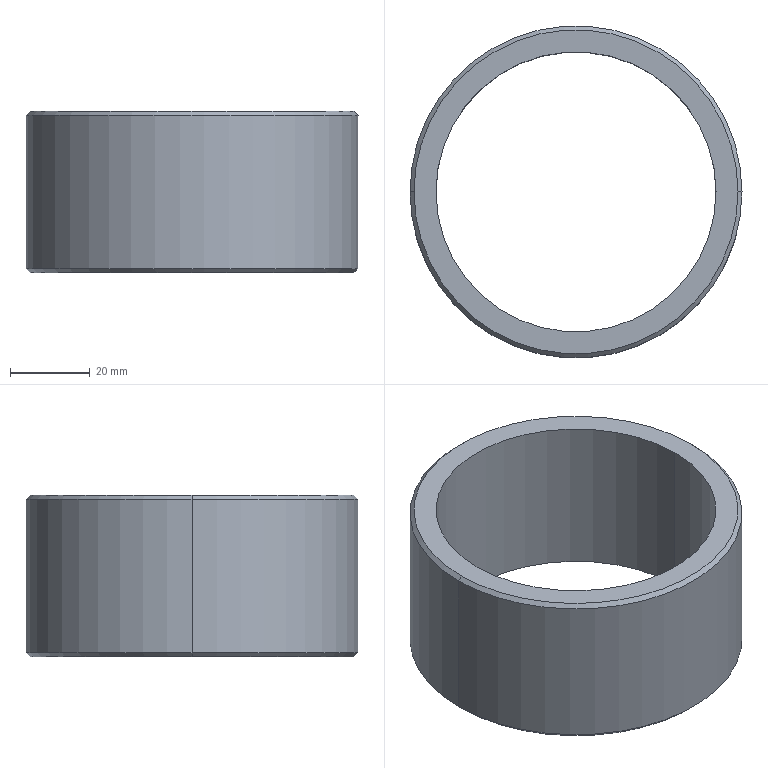Part | SolidWorks | features Chamfer 1, Extrusion 1 | 1 solid | 10 faces | box 83 x 83 x 40.5 mm | volume 63009 mm3 | cone 4 | cylinder 4 | plane 2 | commonest cylinder face diameters 70 x2 83 x2
STEP:
#1=CARTESIAN_POINT('',(40.5,0.,40.5));
#2=VERTEX_POINT('',#1);
#3=CARTESIAN_POINT('',(-40.5,0.,40.5));
#4=VERTEX_POINT('',#3);
#5=CARTESIAN_POINT('',(0.,0.,40.5));
#6=DIRECTION('',(0.,0.,1.));
#7=DIRECTION('',(1.,0.,0.));
#8=AXIS2_PLACEMENT_3D('',#5,#6,#7);
#9=CIRCLE('',#8,40.5);
#10=EDGE_CURVE('',#2,#4,#9,.T.);
#11=ORIENTED_EDGE('',*,*,#10,.F.);
#12=CARTESIAN_POINT('',(41.5,0.,39.5));
#13=VERTEX_POINT('',#12);
#14=CARTESIAN_POINT('',(40.5,0.,40.5));
#15=DIRECTION('',(0.7071,0.,-0.7071));
#16=VECTOR('',#15,1000.);
#17=LINE('',#14,#16);
#18=EDGE_CURVE('',#2,#13,#17,.T.);
#19=ORIENTED_EDGE('',*,*,#18,.T.);
#20=CARTESIAN_POINT('',(-41.5,0.,39.5));
#21=VERTEX_POINT('',#20);
#22=CARTESIAN_POINT('',(0.,0.,39.5));
#23=DIRECTION('',(0.,0.,-1.));
#24=DIRECTION('',(1.,0.,0.));
#25=AXIS2_PLACEMENT_3D('',#22,#23,#24);
#26=CIRCLE('',#25,41.5);
#27=EDGE_CURVE('',#21,#13,#26,.T.);
#28=ORIENTED_EDGE('',*,*,#27,.F.);
#29=CARTESIAN_POINT('',(-40.5,0.,40.5));
#30=DIRECTION('',(-0.7071,0.,-0.7071));
#31=VECTOR('',#30,1000.);
#32=LINE('',#29,#31);
#33=EDGE_CURVE('',#4,#21,#32,.T.);
#34=ORIENTED_EDGE('',*,*,#33,.F.);
#35=EDGE_LOOP('',(#11,#19,#28,#34));
#36=FACE_OUTER_BOUND('',#35,.T.);
#37=CARTESIAN_POINT('',(0.,0.,40.5));
#38=DIRECTION('',(0.,0.,-1.));
#39=DIRECTION('',(-1.,0.,0.));
#40=AXIS2_PLACEMENT_3D('',#37,#38,#39);
#41=CONICAL_SURFACE('',#40,40.5,0.7854);
#42=ADVANCED_FACE('',(#36),#41,.T.);
#43=CARTESIAN_POINT('',(-40.5,0.,0.));
#44=VERTEX_POINT('',#43);
#45=CARTESIAN_POINT('',(40.5,0.,0.));
#46=VERTEX_POINT('',#45);
#47=CARTESIAN_POINT('',(0.,0.,0.));
#48=DIRECTION('',(0.,0.,-1.));
#49=DIRECTION('',(1.,0.,0.));
#50=AXIS2_PLACEMENT_3D('',#47,#48,#49);
#51=CIRCLE('',#50,40.5);
#52=EDGE_CURVE('',#44,#46,#51,.T.);
#53=ORIENTED_EDGE('',*,*,#52,.F.);
#54=CARTESIAN_POINT('',(-41.5,0.,1.));
#55=VERTEX_POINT('',#54);
#56=CARTESIAN_POINT('',(-41.5,0.,1.));
#57=DIRECTION('',(-0.7071,0.,0.7071));
#58=VECTOR('',#57,1000.);
#59=LINE('',#56,#58);
#60=EDGE_CURVE('',#44,#55,#59,.T.);
#61=ORIENTED_EDGE('',*,*,#60,.T.);
#62=CARTESIAN_POINT('',(41.5,0.,1.));
#63=VERTEX_POINT('',#62);
#64=CARTESIAN_POINT('',(0.,0.,1.));
#65=DIRECTION('',(0.,0.,1.));
#66=DIRECTION('',(1.,0.,0.));
#67=AXIS2_PLACEMENT_3D('',#64,#65,#66);
#68=CIRCLE('',#67,41.5);
#69=EDGE_CURVE('',#63,#55,#68,.T.);
#70=ORIENTED_EDGE('',*,*,#69,.F.);
#71=CARTESIAN_POINT('',(41.5,0.,1.));
#72=DIRECTION('',(0.7071,0.,0.7071));
#73=VECTOR('',#72,1000.);
#74=LINE('',#71,#73);
#75=EDGE_CURVE('',#46,#63,#74,.T.);
#76=ORIENTED_EDGE('',*,*,#75,.F.);
#77=EDGE_LOOP('',(#53,#61,#70,#76));
#78=FACE_OUTER_BOUND('',#77,.T.);
#79=CARTESIAN_POINT('',(0.,0.,1.));
#80=DIRECTION('',(0.,0.,1.));
#81=DIRECTION('',(1.,0.,0.));
#82=AXIS2_PLACEMENT_3D('',#79,#80,#81);
#83=CONICAL_SURFACE('',#82,41.5,0.7854);
#84=ADVANCED_FACE('',(#78),#83,.T.);
#85=CARTESIAN_POINT('',(-35.,0.,40.5));
#86=VERTEX_POINT('',#85);
#87=CARTESIAN_POINT('',(35.,0.,40.5));
#88=VERTEX_POINT('',#87);
#89=CARTESIAN_POINT('',(0.,0.,40.5));
#90=DIRECTION('',(0.,0.,1.));
#91=DIRECTION('',(1.,0.,0.));
#92=AXIS2_PLACEMENT_3D('',#89,#90,#91);
#93=CIRCLE('',#92,35.);
#94=EDGE_CURVE('',#86,#88,#93,.T.);
#95=ORIENTED_EDGE('',*,*,#94,.T.);
#96=CARTESIAN_POINT('',(35.,0.,0.));
#97=VERTEX_POINT('',#96);
#98=CARTESIAN_POINT('',(35.,0.,40.5));
#99=DIRECTION('',(0.,0.,-1.));
#100=VECTOR('',#99,1000.);
#101=LINE('',#98,#100);
#102=EDGE_CURVE('',#88,#97,#101,.T.);
#103=ORIENTED_EDGE('',*,*,#102,.T.);
#104=CARTESIAN_POINT('',(-35.,0.,0.));
#105=VERTEX_POINT('',#104);
#106=CARTESIAN_POINT('',(0.,0.,0.));
#107=DIRECTION('',(0.,0.,1.));
#108=DIRECTION('',(1.,0.,0.));
#109=AXIS2_PLACEMENT_3D('',#106,#107,#108);
#110=CIRCLE('',#109,35.);
#111=EDGE_CURVE('',#105,#97,#110,.T.);
#112=ORIENTED_EDGE('',*,*,#111,.F.);
#113=CARTESIAN_POINT('',(-35.,0.,40.5));
#114=DIRECTION('',(0.,0.,-1.));
#115=VECTOR('',#114,1000.);
#116=LINE('',#113,#115);
#117=EDGE_CURVE('',#86,#105,#116,.T.);
#118=ORIENTED_EDGE('',*,*,#117,.F.);
#119=EDGE_LOOP('',(#95,#103,#112,#118));
#120=FACE_OUTER_BOUND('',#119,.T.);
#121=CARTESIAN_POINT('',(0.,0.,40.5));
#122=DIRECTION('',(0.,0.,-1.));
#123=DIRECTION('',(-1.,0.,0.));
#124=AXIS2_PLACEMENT_3D('',#121,#122,#123);
#125=CYLINDRICAL_SURFACE('',#124,35.);
#126=ADVANCED_FACE('',(#120),#125,.F.);
#127=ORIENTED_EDGE('',*,*,#27,.T.);
#128=CARTESIAN_POINT('',(41.5,0.,40.5));
#129=DIRECTION('',(0.,0.,-1.));
#130=VECTOR('',#129,1000.);
#131=LINE('',#128,#130);
#132=EDGE_CURVE('',#13,#63,#131,.T.);
#133=ORIENTED_EDGE('',*,*,#132,.T.);
#134=ORIENTED_EDGE('',*,*,#69,.T.);
#135=CARTESIAN_POINT('',(-41.5,0.,40.5));
#136=DIRECTION('',(0.,0.,-1.));
#137=VECTOR('',#136,1000.);
#138=LINE('',#135,#137);
#139=EDGE_CURVE('',#21,#55,#138,.T.);
#140=ORIENTED_EDGE('',*,*,#139,.F.);
#141=EDGE_LOOP('',(#127,#133,#134,#140));
#142=FACE_OUTER_BOUND('',#141,.T.);
#143=CARTESIAN_POINT('',(0.,0.,40.5));
#144=DIRECTION('',(0.,0.,-1.));
#145=DIRECTION('',(-1.,0.,0.));
#146=AXIS2_PLACEMENT_3D('',#143,#144,#145);
#147=CYLINDRICAL_SURFACE('',#146,41.5);
#148=ADVANCED_FACE('',(#142),#147,.T.);
#149=CARTESIAN_POINT('',(0.,0.,40.5));
#150=DIRECTION('',(0.,0.,1.));
#151=DIRECTION('',(1.,0.,0.));
#152=AXIS2_PLACEMENT_3D('',#149,#150,#151);
#153=CIRCLE('',#152,40.5);
#154=EDGE_CURVE('',#4,#2,#153,.T.);
#155=ORIENTED_EDGE('',*,*,#154,.T.);
#156=ORIENTED_EDGE('',*,*,#10,.T.);
#157=EDGE_LOOP('',(#155,#156));
#158=FACE_OUTER_BOUND('',#157,.T.);
#159=ORIENTED_EDGE('',*,*,#94,.F.);
#160=CARTESIAN_POINT('',(0.,0.,40.5));
#161=DIRECTION('',(0.,0.,1.));
#162=DIRECTION('',(1.,0.,0.));
#163=AXIS2_PLACEMENT_3D('',#160,#161,#162);
#164=CIRCLE('',#163,35.);
#165=EDGE_CURVE('',#88,#86,#164,.T.);
#166=ORIENTED_EDGE('',*,*,#165,.F.);
#167=EDGE_LOOP('',(#159,#166));
#168=FACE_BOUND('',#167,.T.);
#169=CARTESIAN_POINT('',(0.,0.,40.5));
#170=DIRECTION('',(0.,0.,1.));
#171=DIRECTION('',(1.,0.,0.));
#172=AXIS2_PLACEMENT_3D('',#169,#170,#171);
#173=PLANE('',#172);
#174=ADVANCED_FACE('',(#158,#168),#173,.T.);
#175=CARTESIAN_POINT('',(0.,0.,0.));
#176=DIRECTION('',(0.,0.,-1.));
#177=DIRECTION('',(1.,0.,0.));
#178=AXIS2_PLACEMENT_3D('',#175,#176,#177);
#179=CIRCLE('',#178,40.5);
#180=EDGE_CURVE('',#46,#44,#179,.T.);
#181=ORIENTED_EDGE('',*,*,#180,.T.);
#182=ORIENTED_EDGE('',*,*,#52,.T.);
#183=EDGE_LOOP('',(#181,#182));
#184=FACE_OUTER_BOUND('',#183,.T.);
#185=ORIENTED_EDGE('',*,*,#111,.T.);
#186=CARTESIAN_POINT('',(0.,0.,0.));
#187=DIRECTION('',(0.,0.,1.));
#188=DIRECTION('',(1.,0.,0.));
#189=AXIS2_PLACEMENT_3D('',#186,#187,#188);
#190=CIRCLE('',#189,35.);
#191=EDGE_CURVE('',#97,#105,#190,.T.);
#192=ORIENTED_EDGE('',*,*,#191,.T.);
#193=EDGE_LOOP('',(#185,#192));
#194=FACE_BOUND('',#193,.T.);
#195=CARTESIAN_POINT('',(0.,0.,0.));
#196=DIRECTION('',(0.,0.,1.));
#197=DIRECTION('',(1.,0.,0.));
#198=AXIS2_PLACEMENT_3D('',#195,#196,#197);
#199=PLANE('',#198);
#200=ADVANCED_FACE('',(#184,#194),#199,.F.);
#201=ORIENTED_EDGE('',*,*,#132,.F.);
#202=CARTESIAN_POINT('',(0.,0.,39.5));
#203=DIRECTION('',(0.,0.,-1.));
#204=DIRECTION('',(1.,0.,0.));
#205=AXIS2_PLACEMENT_3D('',#202,#203,#204);
#206=CIRCLE('',#205,41.5);
#207=EDGE_CURVE('',#13,#21,#206,.T.);
#208=ORIENTED_EDGE('',*,*,#207,.T.);
#209=ORIENTED_EDGE('',*,*,#139,.T.);
#210=CARTESIAN_POINT('',(0.,0.,1.));
#211=DIRECTION('',(0.,0.,1.));
#212=DIRECTION('',(1.,0.,0.));
#213=AXIS2_PLACEMENT_3D('',#210,#211,#212);
#214=CIRCLE('',#213,41.5);
#215=EDGE_CURVE('',#55,#63,#214,.T.);
#216=ORIENTED_EDGE('',*,*,#215,.T.);
#217=EDGE_LOOP('',(#201,#208,#209,#216));
#218=FACE_OUTER_BOUND('',#217,.T.);
#219=CARTESIAN_POINT('',(0.,0.,40.5));
#220=DIRECTION('',(0.,0.,-1.));
#221=DIRECTION('',(-1.,0.,0.));
#222=AXIS2_PLACEMENT_3D('',#219,#220,#221);
#223=CYLINDRICAL_SURFACE('',#222,41.5);
#224=ADVANCED_FACE('',(#218),#223,.T.);
#225=ORIENTED_EDGE('',*,*,#102,.F.);
#226=ORIENTED_EDGE('',*,*,#165,.T.);
#227=ORIENTED_EDGE('',*,*,#117,.T.);
#228=ORIENTED_EDGE('',*,*,#191,.F.);
#229=EDGE_LOOP('',(#225,#226,#227,#228));
#230=FACE_OUTER_BOUND('',#229,.T.);
#231=CARTESIAN_POINT('',(0.,0.,40.5));
#232=DIRECTION('',(0.,0.,-1.));
#233=DIRECTION('',(-1.,0.,0.));
#234=AXIS2_PLACEMENT_3D('',#231,#232,#233);
#235=CYLINDRICAL_SURFACE('',#234,35.);
#236=ADVANCED_FACE('',(#230),#235,.F.);
#237=ORIENTED_EDGE('',*,*,#60,.F.);
#238=ORIENTED_EDGE('',*,*,#180,.F.);
#239=ORIENTED_EDGE('',*,*,#75,.T.);
#240=ORIENTED_EDGE('',*,*,#215,.F.);
#241=EDGE_LOOP('',(#237,#238,#239,#240));
#242=FACE_OUTER_BOUND('',#241,.T.);
#243=CARTESIAN_POINT('',(0.,0.,1.));
#244=DIRECTION('',(0.,0.,1.));
#245=DIRECTION('',(1.,0.,0.));
#246=AXIS2_PLACEMENT_3D('',#243,#244,#245);
#247=CONICAL_SURFACE('',#246,41.5,0.7854);
#248=ADVANCED_FACE('',(#242),#247,.T.);
#249=ORIENTED_EDGE('',*,*,#18,.F.);
#250=ORIENTED_EDGE('',*,*,#154,.F.);
#251=ORIENTED_EDGE('',*,*,#33,.T.);
#252=ORIENTED_EDGE('',*,*,#207,.F.);
#253=EDGE_LOOP('',(#249,#250,#251,#252));
#254=FACE_OUTER_BOUND('',#253,.T.);
#255=CARTESIAN_POINT('',(0.,0.,40.5));
#256=DIRECTION('',(0.,0.,-1.));
#257=DIRECTION('',(-1.,0.,0.));
#258=AXIS2_PLACEMENT_3D('',#255,#256,#257);
#259=CONICAL_SURFACE('',#258,40.5,0.7854);
#260=ADVANCED_FACE('',(#254),#259,.T.);
#261=CLOSED_SHELL('',(#42,#84,#126,#148,#174,#200,#224,#236,#248,#260));
#262=MANIFOLD_SOLID_BREP('',#261);
#263=CARTESIAN_POINT('',(0.,0.,0.));
#264=DIRECTION('',(0.,0.,1.));
#265=DIRECTION('',(1.,0.,0.));
#266=AXIS2_PLACEMENT_3D('',#263,#264,#265);
#267=(LENGTH_UNIT()NAMED_UNIT(*)SI_UNIT(.MILLI.,.METRE.));
#268=UNCERTAINTY_MEASURE_WITH_UNIT(LENGTH_MEASURE(0.00001),#267,'','');
#269=(NAMED_UNIT(*)PLANE_ANGLE_UNIT()SI_UNIT($,.RADIAN.));
#270=(NAMED_UNIT(*)SI_UNIT($,.STERADIAN.)SOLID_ANGLE_UNIT());
#271=(GEOMETRIC_REPRESENTATION_CONTEXT(3)GLOBAL_UNCERTAINTY_ASSIGNED_CONTEXT((#268))GLOBAL_UNIT_ASSIGNED_CONTEXT((#267,#269,#270))REPRESENTATION_CONTEXT('',''));
#272=ADVANCED_BREP_SHAPE_REPRESENTATION('',(#262,#266),#271);